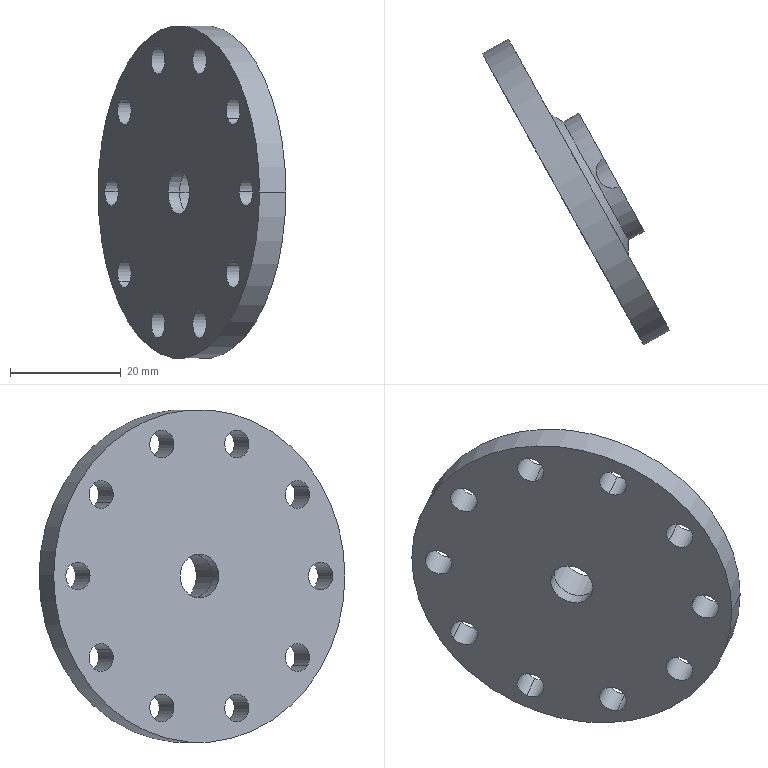Part | STEP file | Completa.sldasm-Part-28_Valor predeterminado | 1 solid | 41 faces | box 33.841 x 55.116 x 60 mm | volume 15153 mm3 | cylinder 32 | plane 4 | torus 3 | cone 2 | commonest cylinder face diameters 5 x20 6 x2 7.936 x2 9.938 x2 24.31 x2 38.784 x2